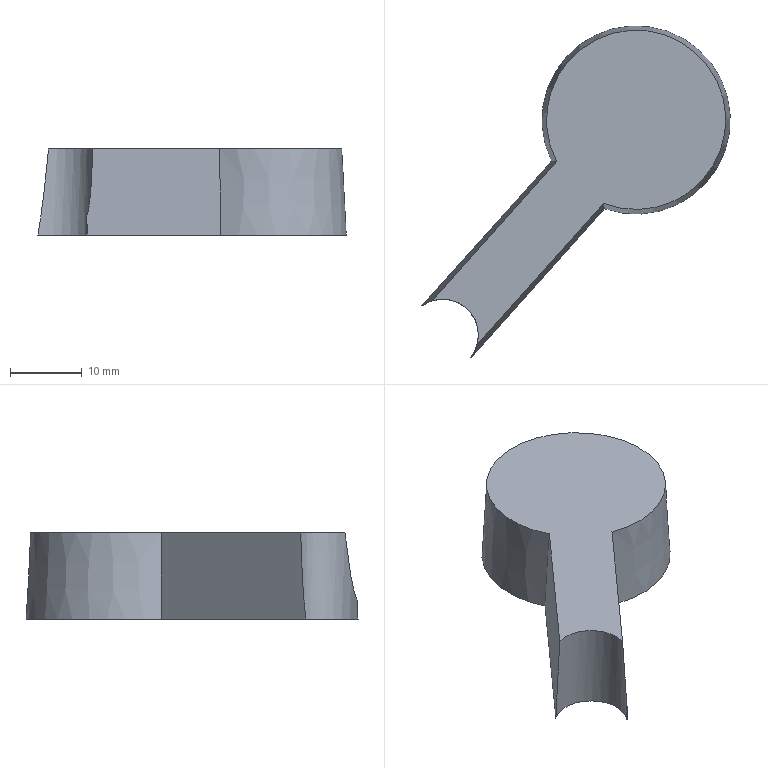Part | STEP file | solid 113 | 1 solid | 7 faces | box 43.011 x 46.317 x 12 mm | volume 8861 mm3 | plane 5 | cone 1 | cylinder 1 | commonest cylinder face diameters 10 x1